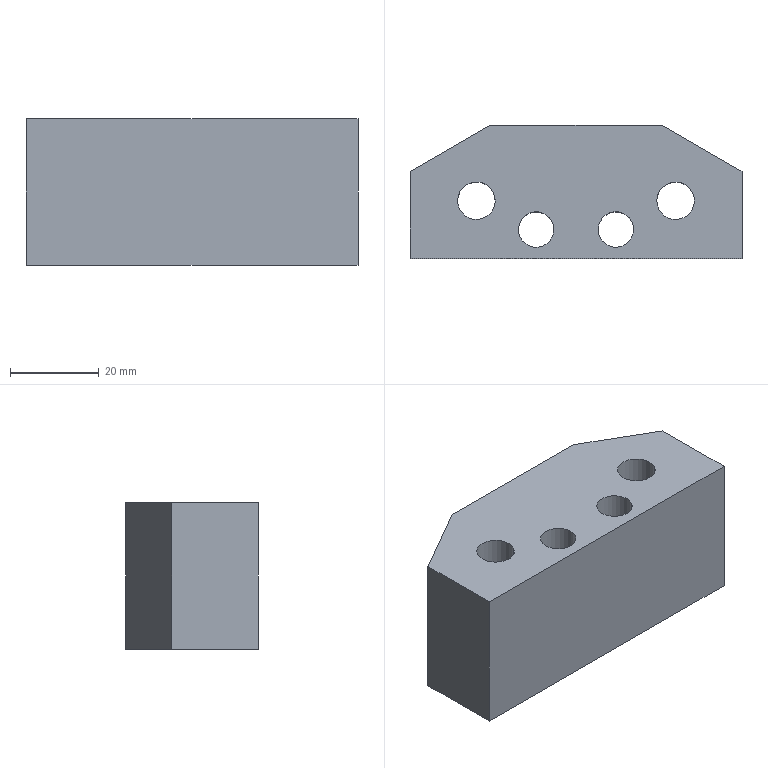Part | CATIA | 1 solid | 16 faces | box 75 x 30 x 33 mm | volume 61014 mm3 | plane 8 | cylinder 8 | commonest cylinder face diameters 8 x4 8.5 x4
STEP:
#1=CARTESIAN_POINT('',(37.5,-30.,38.));
#2=VERTEX_POINT('',#1);
#3=CARTESIAN_POINT('',(37.5,-30.,5.));
#4=VERTEX_POINT('',#3);
#5=CARTESIAN_POINT('',(37.5,-30.,21.5));
#6=DIRECTION('',(0.,0.,-1.));
#7=VECTOR('',#6,1.);
#8=LINE('',#5,#7);
#9=EDGE_CURVE('',#2,#4,#8,.T.);
#10=ORIENTED_EDGE('',*,*,#9,.F.);
#11=CARTESIAN_POINT('',(-37.5,-30.,38.));
#12=VERTEX_POINT('',#11);
#13=CARTESIAN_POINT('',(0.,-30.,38.));
#14=DIRECTION('',(-1.,0.,0.));
#15=VECTOR('',#14,1.);
#16=LINE('',#13,#15);
#17=EDGE_CURVE('',#2,#12,#16,.T.);
#18=ORIENTED_EDGE('',*,*,#17,.T.);
#19=CARTESIAN_POINT('',(-37.5,-30.,5.));
#20=VERTEX_POINT('',#19);
#21=CARTESIAN_POINT('',(-37.5,-30.,21.5));
#22=DIRECTION('',(0.,0.,-1.));
#23=VECTOR('',#22,1.);
#24=LINE('',#21,#23);
#25=EDGE_CURVE('',#12,#20,#24,.T.);
#26=ORIENTED_EDGE('',*,*,#25,.T.);
#27=CARTESIAN_POINT('',(0.,-30.,5.));
#28=DIRECTION('',(-1.,0.,0.));
#29=VECTOR('',#28,1.);
#30=LINE('',#27,#29);
#31=EDGE_CURVE('',#4,#20,#30,.T.);
#32=ORIENTED_EDGE('',*,*,#31,.F.);
#33=EDGE_LOOP('',(#10,#18,#26,#32));
#34=FACE_OUTER_BOUND('',#33,.T.);
#35=CARTESIAN_POINT('',(37.5,-30.,38.));
#36=DIRECTION('',(0.,-1.,0.));
#37=DIRECTION('',(-1.,0.,0.));
#38=AXIS2_PLACEMENT_3D('',#35,#36,#37);
#39=PLANE('',#38);
#40=ADVANCED_FACE('',(#34),#39,.T.);
#41=CARTESIAN_POINT('',(-37.5,-10.392,38.));
#42=VERTEX_POINT('',#41);
#43=CARTESIAN_POINT('',(-37.5,-10.392,5.));
#44=VERTEX_POINT('',#43);
#45=CARTESIAN_POINT('',(-37.5,-10.392,21.5));
#46=DIRECTION('',(0.,0.,-1.));
#47=VECTOR('',#46,1.);
#48=LINE('',#45,#47);
#49=EDGE_CURVE('',#42,#44,#48,.T.);
#50=ORIENTED_EDGE('',*,*,#49,.T.);
#51=CARTESIAN_POINT('',(-37.5,-20.196,5.));
#52=DIRECTION('',(0.,-1.,0.));
#53=VECTOR('',#52,1.);
#54=LINE('',#51,#53);
#55=EDGE_CURVE('',#20,#44,#54,.F.);
#56=ORIENTED_EDGE('',*,*,#55,.F.);
#57=ORIENTED_EDGE('',*,*,#25,.F.);
#58=CARTESIAN_POINT('',(-37.5,-20.196,38.));
#59=DIRECTION('',(0.,-1.,0.));
#60=VECTOR('',#59,1.);
#61=LINE('',#58,#60);
#62=EDGE_CURVE('',#12,#42,#61,.F.);
#63=ORIENTED_EDGE('',*,*,#62,.T.);
#64=EDGE_LOOP('',(#50,#56,#57,#63));
#65=FACE_OUTER_BOUND('',#64,.T.);
#66=CARTESIAN_POINT('',(-37.5,0.,38.));
#67=DIRECTION('',(1.,0.,0.));
#68=DIRECTION('',(0.,-1.,0.));
#69=AXIS2_PLACEMENT_3D('',#66,#67,#68);
#70=PLANE('',#69);
#71=ADVANCED_FACE('',(#65),#70,.F.);
#72=CARTESIAN_POINT('',(-19.5,0.,5.));
#73=VERTEX_POINT('',#72);
#74=CARTESIAN_POINT('',(-28.5,-5.196,5.));
#75=DIRECTION('',(-0.866,-0.5,0.));
#76=VECTOR('',#75,1.);
#77=LINE('',#74,#76);
#78=EDGE_CURVE('',#73,#44,#77,.T.);
#79=ORIENTED_EDGE('',*,*,#78,.T.);
#80=ORIENTED_EDGE('',*,*,#49,.F.);
#81=CARTESIAN_POINT('',(-19.5,0.,38.));
#82=VERTEX_POINT('',#81);
#83=CARTESIAN_POINT('',(-28.5,-5.196,38.));
#84=DIRECTION('',(-0.866,-0.5,0.));
#85=VECTOR('',#84,1.);
#86=LINE('',#83,#85);
#87=EDGE_CURVE('',#42,#82,#86,.F.);
#88=ORIENTED_EDGE('',*,*,#87,.T.);
#89=CARTESIAN_POINT('',(-19.5,0.,21.5));
#90=DIRECTION('',(0.,0.,-1.));
#91=VECTOR('',#90,1.);
#92=LINE('',#89,#91);
#93=EDGE_CURVE('',#82,#73,#92,.T.);
#94=ORIENTED_EDGE('',*,*,#93,.T.);
#95=EDGE_LOOP('',(#79,#80,#88,#94));
#96=FACE_OUTER_BOUND('',#95,.T.);
#97=CARTESIAN_POINT('',(-19.5,0.,44.6));
#98=DIRECTION('',(-0.5,0.866,0.));
#99=DIRECTION('',(0.,0.,-1.));
#100=AXIS2_PLACEMENT_3D('',#97,#98,#99);
#101=PLANE('',#100);
#102=ADVANCED_FACE('',(#96),#101,.T.);
#103=CARTESIAN_POINT('',(37.5,-10.392,38.));
#104=VERTEX_POINT('',#103);
#105=CARTESIAN_POINT('',(37.5,-10.392,5.));
#106=VERTEX_POINT('',#105);
#107=CARTESIAN_POINT('',(37.5,-10.392,21.5));
#108=DIRECTION('',(0.,0.,1.));
#109=VECTOR('',#108,1.);
#110=LINE('',#107,#109);
#111=EDGE_CURVE('',#104,#106,#110,.F.);
#112=ORIENTED_EDGE('',*,*,#111,.F.);
#113=CARTESIAN_POINT('',(37.5,-20.196,38.));
#114=DIRECTION('',(0.,1.,0.));
#115=VECTOR('',#114,1.);
#116=LINE('',#113,#115);
#117=EDGE_CURVE('',#104,#2,#116,.F.);
#118=ORIENTED_EDGE('',*,*,#117,.T.);
#119=ORIENTED_EDGE('',*,*,#9,.T.);
#120=CARTESIAN_POINT('',(37.5,-20.196,5.));
#121=DIRECTION('',(0.,1.,0.));
#122=VECTOR('',#121,1.);
#123=LINE('',#120,#122);
#124=EDGE_CURVE('',#106,#4,#123,.F.);
#125=ORIENTED_EDGE('',*,*,#124,.F.);
#126=EDGE_LOOP('',(#112,#118,#119,#125));
#127=FACE_OUTER_BOUND('',#126,.T.);
#128=CARTESIAN_POINT('',(37.5,-30.,38.));
#129=DIRECTION('',(-1.,0.,0.));
#130=DIRECTION('',(0.,1.,0.));
#131=AXIS2_PLACEMENT_3D('',#128,#129,#130);
#132=PLANE('',#131);
#133=ADVANCED_FACE('',(#127),#132,.F.);
#134=CARTESIAN_POINT('',(19.5,0.,5.));
#135=VERTEX_POINT('',#134);
#136=CARTESIAN_POINT('',(0.,0.,5.));
#137=DIRECTION('',(1.,0.,0.));
#138=VECTOR('',#137,1.);
#139=LINE('',#136,#138);
#140=EDGE_CURVE('',#73,#135,#139,.T.);
#141=ORIENTED_EDGE('',*,*,#140,.F.);
#142=ORIENTED_EDGE('',*,*,#93,.F.);
#143=CARTESIAN_POINT('',(19.5,0.,38.));
#144=VERTEX_POINT('',#143);
#145=CARTESIAN_POINT('',(0.,0.,38.));
#146=DIRECTION('',(1.,0.,0.));
#147=VECTOR('',#146,1.);
#148=LINE('',#145,#147);
#149=EDGE_CURVE('',#82,#144,#148,.T.);
#150=ORIENTED_EDGE('',*,*,#149,.T.);
#151=CARTESIAN_POINT('',(19.5,0.,21.5));
#152=DIRECTION('',(0.,0.,1.));
#153=VECTOR('',#152,1.);
#154=LINE('',#151,#153);
#155=EDGE_CURVE('',#144,#135,#154,.F.);
#156=ORIENTED_EDGE('',*,*,#155,.T.);
#157=EDGE_LOOP('',(#141,#142,#150,#156));
#158=FACE_OUTER_BOUND('',#157,.T.);
#159=CARTESIAN_POINT('',(-37.5,0.,38.));
#160=DIRECTION('',(0.,1.,0.));
#161=DIRECTION('',(1.,0.,0.));
#162=AXIS2_PLACEMENT_3D('',#159,#160,#161);
#163=PLANE('',#162);
#164=ADVANCED_FACE('',(#158),#163,.T.);
#165=CARTESIAN_POINT('',(28.5,-5.196,5.));
#166=DIRECTION('',(0.866,-0.5,0.));
#167=VECTOR('',#166,1.);
#168=LINE('',#165,#167);
#169=EDGE_CURVE('',#106,#135,#168,.F.);
#170=ORIENTED_EDGE('',*,*,#169,.T.);
#171=ORIENTED_EDGE('',*,*,#155,.F.);
#172=CARTESIAN_POINT('',(28.5,-5.196,38.));
#173=DIRECTION('',(0.866,-0.5,0.));
#174=VECTOR('',#173,1.);
#175=LINE('',#172,#174);
#176=EDGE_CURVE('',#144,#104,#175,.T.);
#177=ORIENTED_EDGE('',*,*,#176,.T.);
#178=ORIENTED_EDGE('',*,*,#111,.T.);
#179=EDGE_LOOP('',(#170,#171,#177,#178));
#180=FACE_OUTER_BOUND('',#179,.T.);
#181=CARTESIAN_POINT('',(19.5,0.,-1.6));
#182=DIRECTION('',(0.5,0.866,0.));
#183=DIRECTION('',(0.,0.,1.));
#184=AXIS2_PLACEMENT_3D('',#181,#182,#183);
#185=PLANE('',#184);
#186=ADVANCED_FACE('',(#180),#185,.T.);
#187=ORIENTED_EDGE('',*,*,#124,.T.);
#188=ORIENTED_EDGE('',*,*,#31,.T.);
#189=ORIENTED_EDGE('',*,*,#55,.T.);
#190=ORIENTED_EDGE('',*,*,#78,.F.);
#191=ORIENTED_EDGE('',*,*,#140,.T.);
#192=ORIENTED_EDGE('',*,*,#169,.F.);
#193=EDGE_LOOP('',(#187,#188,#189,#190,#191,#192));
#194=FACE_OUTER_BOUND('',#193,.T.);
#195=CARTESIAN_POINT('',(-26.23,-14.962,5.));
#196=VERTEX_POINT('',#195);
#197=CARTESIAN_POINT('',(-18.77,-19.038,5.));
#198=VERTEX_POINT('',#197);
#199=CARTESIAN_POINT('',(-22.5,-17.,5.));
#200=DIRECTION('',(0.,0.,-1.));
#201=AXIS2_PLACEMENT_3D('',#199,#200,$);
#202=CIRCLE('',#201,4.25);
#203=EDGE_CURVE('',#196,#198,#202,.T.);
#204=ORIENTED_EDGE('',*,*,#203,.F.);
#205=CARTESIAN_POINT('',(-22.5,-17.,5.));
#206=DIRECTION('',(0.,0.,-1.));
#207=AXIS2_PLACEMENT_3D('',#205,#206,$);
#208=CIRCLE('',#207,4.25);
#209=EDGE_CURVE('',#198,#196,#208,.T.);
#210=ORIENTED_EDGE('',*,*,#209,.F.);
#211=EDGE_LOOP('',(#204,#210));
#212=FACE_BOUND('',#211,.T.);
#213=CARTESIAN_POINT('',(18.77,-14.962,5.));
#214=VERTEX_POINT('',#213);
#215=CARTESIAN_POINT('',(26.23,-19.038,5.));
#216=VERTEX_POINT('',#215);
#217=CARTESIAN_POINT('',(22.5,-17.,5.));
#218=DIRECTION('',(0.,0.,-1.));
#219=AXIS2_PLACEMENT_3D('',#217,#218,$);
#220=CIRCLE('',#219,4.25);
#221=EDGE_CURVE('',#214,#216,#220,.T.);
#222=ORIENTED_EDGE('',*,*,#221,.F.);
#223=CARTESIAN_POINT('',(22.5,-17.,5.));
#224=DIRECTION('',(0.,0.,-1.));
#225=AXIS2_PLACEMENT_3D('',#223,#224,$);
#226=CIRCLE('',#225,4.25);
#227=EDGE_CURVE('',#216,#214,#226,.T.);
#228=ORIENTED_EDGE('',*,*,#227,.F.);
#229=EDGE_LOOP('',(#222,#228));
#230=FACE_BOUND('',#229,.T.);
#231=CARTESIAN_POINT('',(-12.51,-21.582,5.));
#232=VERTEX_POINT('',#231);
#233=CARTESIAN_POINT('',(-5.49,-25.418,5.));
#234=VERTEX_POINT('',#233);
#235=CARTESIAN_POINT('',(-9.,-23.5,5.));
#236=DIRECTION('',(0.,0.,-1.));
#237=AXIS2_PLACEMENT_3D('',#235,#236,$);
#238=CIRCLE('',#237,4.);
#239=EDGE_CURVE('',#232,#234,#238,.T.);
#240=ORIENTED_EDGE('',*,*,#239,.F.);
#241=CARTESIAN_POINT('',(-9.,-23.5,5.));
#242=DIRECTION('',(0.,0.,-1.));
#243=AXIS2_PLACEMENT_3D('',#241,#242,$);
#244=CIRCLE('',#243,4.);
#245=EDGE_CURVE('',#234,#232,#244,.T.);
#246=ORIENTED_EDGE('',*,*,#245,.F.);
#247=EDGE_LOOP('',(#240,#246));
#248=FACE_BOUND('',#247,.T.);
#249=CARTESIAN_POINT('',(5.49,-21.582,5.));
#250=VERTEX_POINT('',#249);
#251=CARTESIAN_POINT('',(12.51,-25.418,5.));
#252=VERTEX_POINT('',#251);
#253=CARTESIAN_POINT('',(9.,-23.5,5.));
#254=DIRECTION('',(0.,0.,-1.));
#255=AXIS2_PLACEMENT_3D('',#253,#254,$);
#256=CIRCLE('',#255,4.);
#257=EDGE_CURVE('',#250,#252,#256,.T.);
#258=ORIENTED_EDGE('',*,*,#257,.F.);
#259=CARTESIAN_POINT('',(9.,-23.5,5.));
#260=DIRECTION('',(0.,0.,-1.));
#261=AXIS2_PLACEMENT_3D('',#259,#260,$);
#262=CIRCLE('',#261,4.);
#263=EDGE_CURVE('',#252,#250,#262,.T.);
#264=ORIENTED_EDGE('',*,*,#263,.F.);
#265=EDGE_LOOP('',(#258,#264));
#266=FACE_BOUND('',#265,.T.);
#267=CARTESIAN_POINT('',(0.,0.,5.));
#268=DIRECTION('',(0.,0.,-1.));
#269=DIRECTION('',(1.,0.,0.));
#270=AXIS2_PLACEMENT_3D('',#267,#268,#269);
#271=PLANE('',#270);
#272=ADVANCED_FACE('',(#194,#212,#230,#248,#266),#271,.T.);
#273=ORIENTED_EDGE('',*,*,#176,.F.);
#274=ORIENTED_EDGE('',*,*,#149,.F.);
#275=ORIENTED_EDGE('',*,*,#87,.F.);
#276=ORIENTED_EDGE('',*,*,#62,.F.);
#277=ORIENTED_EDGE('',*,*,#17,.F.);
#278=ORIENTED_EDGE('',*,*,#117,.F.);
#279=EDGE_LOOP('',(#273,#274,#275,#276,#277,#278));
#280=FACE_OUTER_BOUND('',#279,.T.);
#281=CARTESIAN_POINT('',(-26.23,-14.962,38.));
#282=VERTEX_POINT('',#281);
#283=CARTESIAN_POINT('',(-18.77,-19.038,38.));
#284=VERTEX_POINT('',#283);
#285=CARTESIAN_POINT('',(-22.5,-17.,38.));
#286=DIRECTION('',(0.,0.,-1.));
#287=AXIS2_PLACEMENT_3D('',#285,#286,$);
#288=CIRCLE('',#287,4.25);
#289=EDGE_CURVE('',#282,#284,#288,.T.);
#290=ORIENTED_EDGE('',*,*,#289,.T.);
#291=CARTESIAN_POINT('',(-22.5,-17.,38.));
#292=DIRECTION('',(0.,0.,-1.));
#293=AXIS2_PLACEMENT_3D('',#291,#292,$);
#294=CIRCLE('',#293,4.25);
#295=EDGE_CURVE('',#284,#282,#294,.T.);
#296=ORIENTED_EDGE('',*,*,#295,.T.);
#297=EDGE_LOOP('',(#290,#296));
#298=FACE_BOUND('',#297,.T.);
#299=CARTESIAN_POINT('',(18.77,-14.962,38.));
#300=VERTEX_POINT('',#299);
#301=CARTESIAN_POINT('',(26.23,-19.038,38.));
#302=VERTEX_POINT('',#301);
#303=CARTESIAN_POINT('',(22.5,-17.,38.));
#304=DIRECTION('',(0.,0.,-1.));
#305=AXIS2_PLACEMENT_3D('',#303,#304,$);
#306=CIRCLE('',#305,4.25);
#307=EDGE_CURVE('',#300,#302,#306,.T.);
#308=ORIENTED_EDGE('',*,*,#307,.T.);
#309=CARTESIAN_POINT('',(22.5,-17.,38.));
#310=DIRECTION('',(0.,0.,-1.));
#311=AXIS2_PLACEMENT_3D('',#309,#310,$);
#312=CIRCLE('',#311,4.25);
#313=EDGE_CURVE('',#302,#300,#312,.T.);
#314=ORIENTED_EDGE('',*,*,#313,.T.);
#315=EDGE_LOOP('',(#308,#314));
#316=FACE_BOUND('',#315,.T.);
#317=CARTESIAN_POINT('',(-12.51,-21.582,38.));
#318=VERTEX_POINT('',#317);
#319=CARTESIAN_POINT('',(-5.49,-25.418,38.));
#320=VERTEX_POINT('',#319);
#321=CARTESIAN_POINT('',(-9.,-23.5,38.));
#322=DIRECTION('',(0.,0.,-1.));
#323=AXIS2_PLACEMENT_3D('',#321,#322,$);
#324=CIRCLE('',#323,4.);
#325=EDGE_CURVE('',#318,#320,#324,.T.);
#326=ORIENTED_EDGE('',*,*,#325,.T.);
#327=CARTESIAN_POINT('',(-9.,-23.5,38.));
#328=DIRECTION('',(0.,0.,-1.));
#329=AXIS2_PLACEMENT_3D('',#327,#328,$);
#330=CIRCLE('',#329,4.);
#331=EDGE_CURVE('',#320,#318,#330,.T.);
#332=ORIENTED_EDGE('',*,*,#331,.T.);
#333=EDGE_LOOP('',(#326,#332));
#334=FACE_BOUND('',#333,.T.);
#335=CARTESIAN_POINT('',(5.49,-21.582,38.));
#336=VERTEX_POINT('',#335);
#337=CARTESIAN_POINT('',(12.51,-25.418,38.));
#338=VERTEX_POINT('',#337);
#339=CARTESIAN_POINT('',(9.,-23.5,38.));
#340=DIRECTION('',(0.,0.,-1.));
#341=AXIS2_PLACEMENT_3D('',#339,#340,$);
#342=CIRCLE('',#341,4.);
#343=EDGE_CURVE('',#336,#338,#342,.T.);
#344=ORIENTED_EDGE('',*,*,#343,.T.);
#345=CARTESIAN_POINT('',(9.,-23.5,38.));
#346=DIRECTION('',(0.,0.,-1.));
#347=AXIS2_PLACEMENT_3D('',#345,#346,$);
#348=CIRCLE('',#347,4.);
#349=EDGE_CURVE('',#338,#336,#348,.T.);
#350=ORIENTED_EDGE('',*,*,#349,.T.);
#351=EDGE_LOOP('',(#344,#350));
#352=FACE_BOUND('',#351,.T.);
#353=CARTESIAN_POINT('',(0.,0.,38.));
#354=DIRECTION('',(0.,0.,-1.));
#355=DIRECTION('',(1.,0.,0.));
#356=AXIS2_PLACEMENT_3D('',#353,#354,#355);
#357=PLANE('',#356);
#358=ADVANCED_FACE('',(#280,#298,#316,#334,#352),#357,.F.);
#359=ORIENTED_EDGE('',*,*,#331,.F.);
#360=CARTESIAN_POINT('',(-5.49,-25.418,21.5));
#361=DIRECTION('',(0.,0.,-1.));
#362=VECTOR('',#361,1.);
#363=LINE('',#360,#362);
#364=EDGE_CURVE('',#234,#320,#363,.F.);
#365=ORIENTED_EDGE('',*,*,#364,.F.);
#366=ORIENTED_EDGE('',*,*,#245,.T.);
#367=CARTESIAN_POINT('',(-12.51,-21.582,21.5));
#368=DIRECTION('',(0.,0.,-1.));
#369=VECTOR('',#368,1.);
#370=LINE('',#367,#369);
#371=EDGE_CURVE('',#232,#318,#370,.F.);
#372=ORIENTED_EDGE('',*,*,#371,.T.);
#373=EDGE_LOOP('',(#359,#365,#366,#372));
#374=FACE_OUTER_BOUND('',#373,.T.);
#375=CARTESIAN_POINT('',(-9.,-23.5,37.9));
#376=DIRECTION('',(0.,0.,-1.));
#377=DIRECTION('',(0.8776,-0.4794,0.));
#378=AXIS2_PLACEMENT_3D('',#375,#376,#377);
#379=CYLINDRICAL_SURFACE('',#378,4.);
#380=ADVANCED_FACE('',(#374),#379,.F.);
#381=ORIENTED_EDGE('',*,*,#325,.F.);
#382=ORIENTED_EDGE('',*,*,#371,.F.);
#383=ORIENTED_EDGE('',*,*,#239,.T.);
#384=ORIENTED_EDGE('',*,*,#364,.T.);
#385=EDGE_LOOP('',(#381,#382,#383,#384));
#386=FACE_OUTER_BOUND('',#385,.T.);
#387=ADVANCED_FACE('',(#386),#379,.F.);
#388=ORIENTED_EDGE('',*,*,#313,.F.);
#389=CARTESIAN_POINT('',(26.23,-19.038,21.5));
#390=DIRECTION('',(0.,0.,-1.));
#391=VECTOR('',#390,1.);
#392=LINE('',#389,#391);
#393=EDGE_CURVE('',#216,#302,#392,.F.);
#394=ORIENTED_EDGE('',*,*,#393,.F.);
#395=ORIENTED_EDGE('',*,*,#227,.T.);
#396=CARTESIAN_POINT('',(18.77,-14.962,21.5));
#397=DIRECTION('',(0.,0.,-1.));
#398=VECTOR('',#397,1.);
#399=LINE('',#396,#398);
#400=EDGE_CURVE('',#214,#300,#399,.F.);
#401=ORIENTED_EDGE('',*,*,#400,.T.);
#402=EDGE_LOOP('',(#388,#394,#395,#401));
#403=FACE_OUTER_BOUND('',#402,.T.);
#404=CARTESIAN_POINT('',(22.5,-17.,37.9));
#405=DIRECTION('',(0.,0.,-1.));
#406=DIRECTION('',(0.8776,-0.4794,0.));
#407=AXIS2_PLACEMENT_3D('',#404,#405,#406);
#408=CYLINDRICAL_SURFACE('',#407,4.25);
#409=ADVANCED_FACE('',(#403),#408,.F.);
#410=ORIENTED_EDGE('',*,*,#307,.F.);
#411=ORIENTED_EDGE('',*,*,#400,.F.);
#412=ORIENTED_EDGE('',*,*,#221,.T.);
#413=ORIENTED_EDGE('',*,*,#393,.T.);
#414=EDGE_LOOP('',(#410,#411,#412,#413));
#415=FACE_OUTER_BOUND('',#414,.T.);
#416=ADVANCED_FACE('',(#415),#408,.F.);
#417=ORIENTED_EDGE('',*,*,#349,.F.);
#418=CARTESIAN_POINT('',(12.51,-25.418,21.5));
#419=DIRECTION('',(0.,0.,-1.));
#420=VECTOR('',#419,1.);
#421=LINE('',#418,#420);
#422=EDGE_CURVE('',#252,#338,#421,.F.);
#423=ORIENTED_EDGE('',*,*,#422,.F.);
#424=ORIENTED_EDGE('',*,*,#263,.T.);
#425=CARTESIAN_POINT('',(5.49,-21.582,21.5));
#426=DIRECTION('',(0.,0.,-1.));
#427=VECTOR('',#426,1.);
#428=LINE('',#425,#427);
#429=EDGE_CURVE('',#250,#336,#428,.F.);
#430=ORIENTED_EDGE('',*,*,#429,.T.);
#431=EDGE_LOOP('',(#417,#423,#424,#430));
#432=FACE_OUTER_BOUND('',#431,.T.);
#433=CARTESIAN_POINT('',(9.,-23.5,37.9));
#434=DIRECTION('',(0.,0.,-1.));
#435=DIRECTION('',(0.8776,-0.4794,0.));
#436=AXIS2_PLACEMENT_3D('',#433,#434,#435);
#437=CYLINDRICAL_SURFACE('',#436,4.);
#438=ADVANCED_FACE('',(#432),#437,.F.);
#439=ORIENTED_EDGE('',*,*,#343,.F.);
#440=ORIENTED_EDGE('',*,*,#429,.F.);
#441=ORIENTED_EDGE('',*,*,#257,.T.);
#442=ORIENTED_EDGE('',*,*,#422,.T.);
#443=EDGE_LOOP('',(#439,#440,#441,#442));
#444=FACE_OUTER_BOUND('',#443,.T.);
#445=ADVANCED_FACE('',(#444),#437,.F.);
#446=ORIENTED_EDGE('',*,*,#295,.F.);
#447=CARTESIAN_POINT('',(-18.77,-19.038,21.5));
#448=DIRECTION('',(0.,0.,-1.));
#449=VECTOR('',#448,1.);
#450=LINE('',#447,#449);
#451=EDGE_CURVE('',#198,#284,#450,.F.);
#452=ORIENTED_EDGE('',*,*,#451,.F.);
#453=ORIENTED_EDGE('',*,*,#209,.T.);
#454=CARTESIAN_POINT('',(-26.23,-14.962,21.5));
#455=DIRECTION('',(0.,0.,-1.));
#456=VECTOR('',#455,1.);
#457=LINE('',#454,#456);
#458=EDGE_CURVE('',#196,#282,#457,.F.);
#459=ORIENTED_EDGE('',*,*,#458,.T.);
#460=EDGE_LOOP('',(#446,#452,#453,#459));
#461=FACE_OUTER_BOUND('',#460,.T.);
#462=CARTESIAN_POINT('',(-22.5,-17.,37.9));
#463=DIRECTION('',(0.,0.,-1.));
#464=DIRECTION('',(0.8776,-0.4794,0.));
#465=AXIS2_PLACEMENT_3D('',#462,#463,#464);
#466=CYLINDRICAL_SURFACE('',#465,4.25);
#467=ADVANCED_FACE('',(#461),#466,.F.);
#468=ORIENTED_EDGE('',*,*,#289,.F.);
#469=ORIENTED_EDGE('',*,*,#458,.F.);
#470=ORIENTED_EDGE('',*,*,#203,.T.);
#471=ORIENTED_EDGE('',*,*,#451,.T.);
#472=EDGE_LOOP('',(#468,#469,#470,#471));
#473=FACE_OUTER_BOUND('',#472,.T.);
#474=ADVANCED_FACE('',(#473),#466,.F.);
#475=CLOSED_SHELL('',(#40,#71,#102,#133,#164,#186,#272,#358,#380,#387,#409,#416,#438,#445,#467,#474));
#476=MANIFOLD_SOLID_BREP('',#475);
#477=(LENGTH_UNIT()NAMED_UNIT(*)SI_UNIT(.MILLI.,.METRE.));
#478=UNCERTAINTY_MEASURE_WITH_UNIT(LENGTH_MEASURE(0.005),#477,'','');
#479=(NAMED_UNIT(*)PLANE_ANGLE_UNIT()SI_UNIT($,.RADIAN.));
#480=(NAMED_UNIT(*)SI_UNIT($,.STERADIAN.)SOLID_ANGLE_UNIT());
#481=(GEOMETRIC_REPRESENTATION_CONTEXT(3)GLOBAL_UNCERTAINTY_ASSIGNED_CONTEXT((#478))GLOBAL_UNIT_ASSIGNED_CONTEXT((#477,#479,#480))REPRESENTATION_CONTEXT('',''));
#482=ADVANCED_BREP_SHAPE_REPRESENTATION('',(#476),#481);